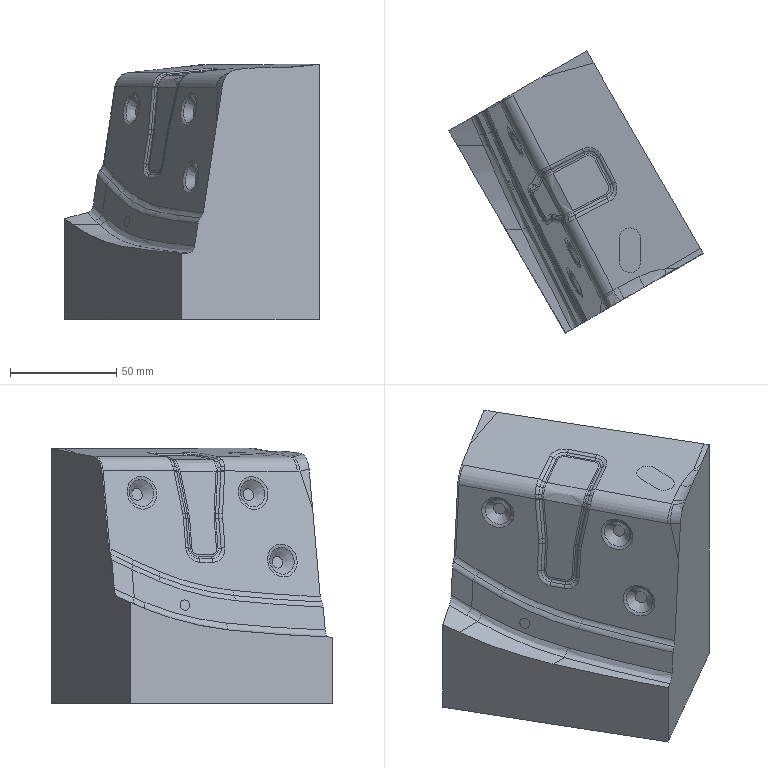Part | NX | features solid 2 | 1 solid | 108 faces | box 119.952 x 132.763 x 120.399 mm | volume 804137 mm3 | spline 103 | plane 5